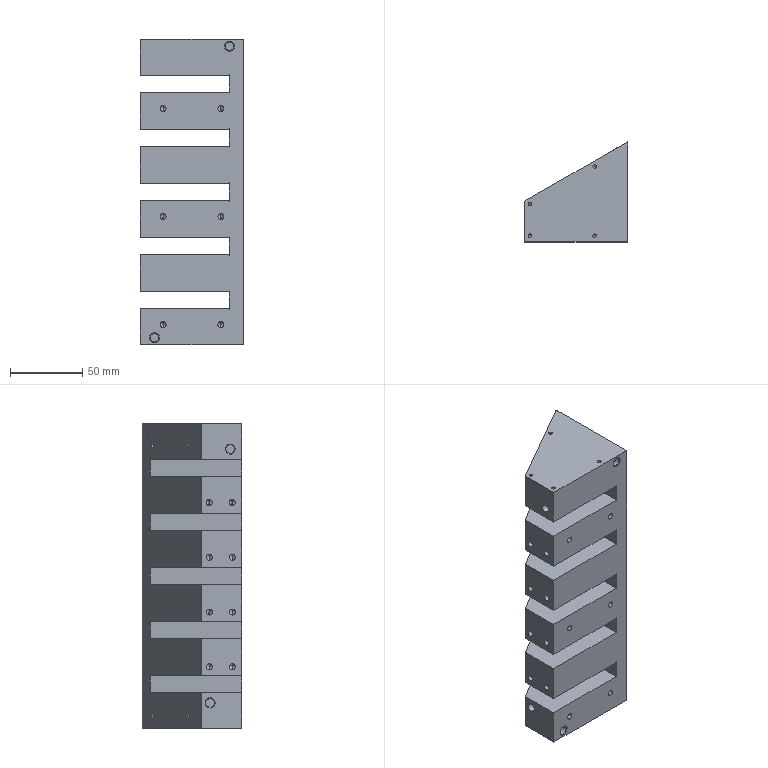Part | STEP file | GLSJ-10-25_default | 1 solid | 202 faces | box 72 x 69 x 212 mm | volume 565884 mm3 | cylinder 91 | cone 76 | plane 35 | commonest cylinder face diameters 2.5 x32 4.2 x28 0.5 x15 3.3 x8 6 x8